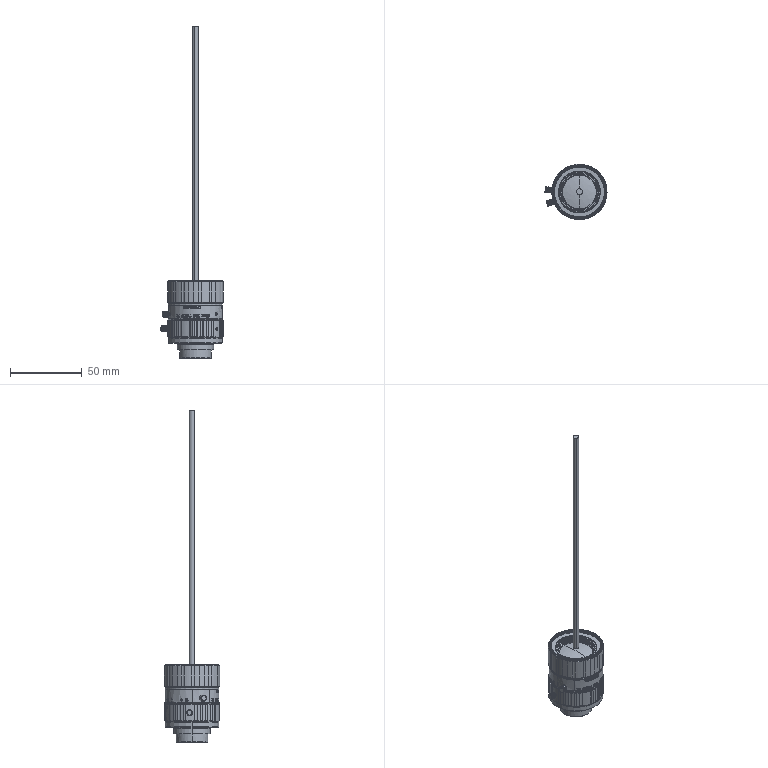Part | SolidWorks | 14 solids | 4651 faces | volume 52174 mm3 | plane 3536 | cylinder 693 | spline 222 | cone 200 | commonest cylinder face diameters 1.6 x153 4 x70 37.5 x57 1.201 x49 38.6 x43 2 x35